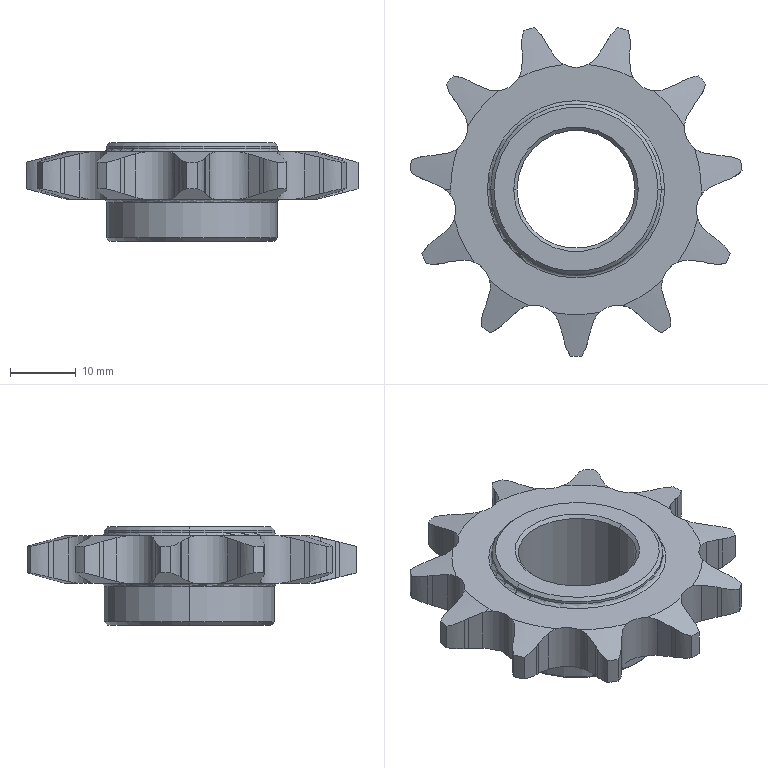Part | STEP file | 04-Small sprocket 2 | 1 solid | 134 faces | box 50.563 x 50.061 x 15 mm | volume 10157 mm3 | cylinder 72 | cone 32 | plane 26 | torus 4 | commonest cylinder face diameters 13.48 x22 20.647 x22 7.967 x11 50.872 x11 26 x4 18 x2